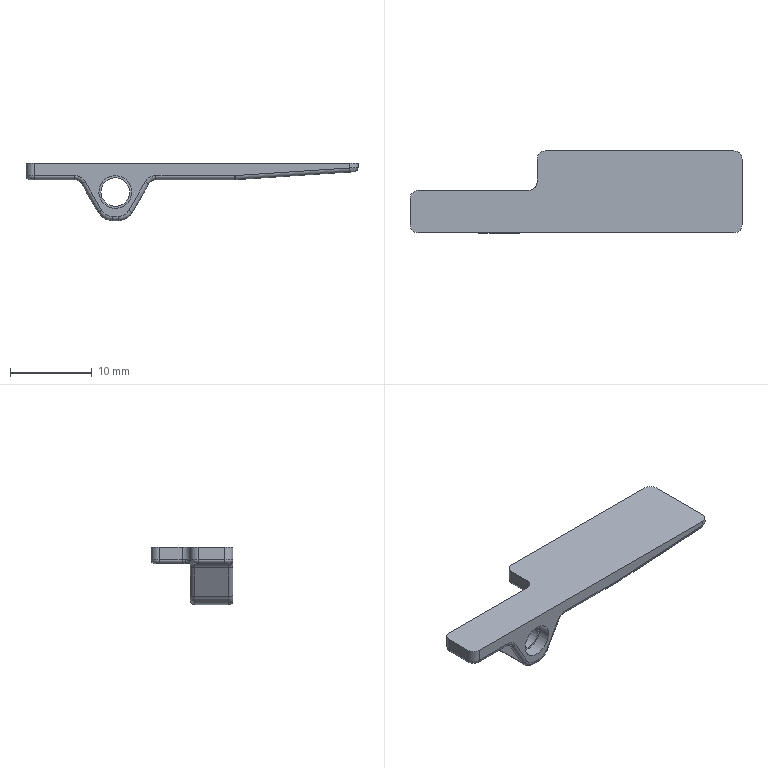Part | 1 solid | 61 faces | box 40.5 x 10 x 7 mm | volume 676.123 mm3 | cylinder 30 | plane 14 | torus 13 | spline 4 | commonest cylinder face diameters 1 x15 2 x9 4 x4 3.5 x2